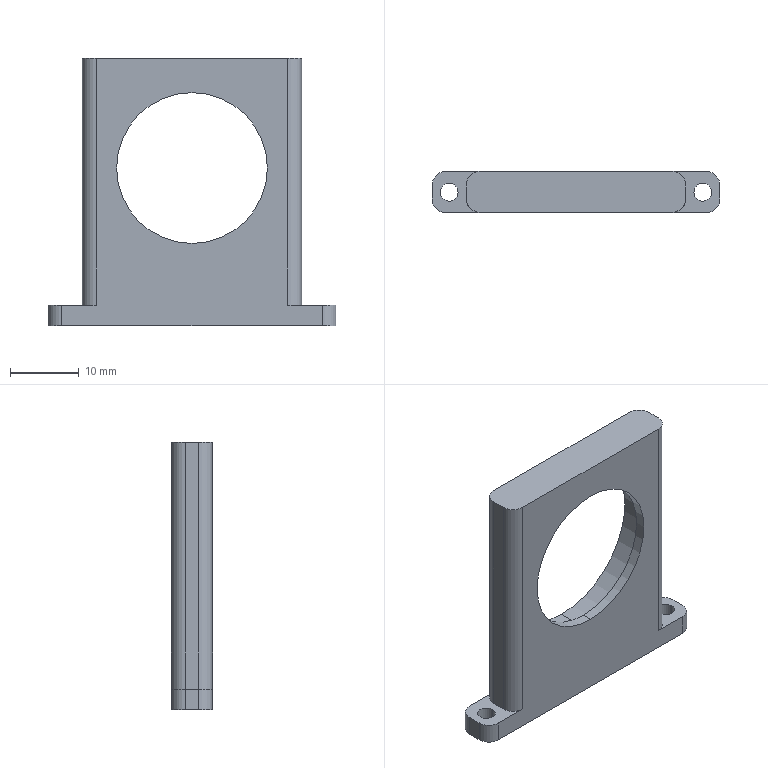NC program | NX | posted with a generic post | part box 42 x 6 x 39 mm
Whole program:
N10 G17 G21 G94 G90
(FLOOR_WALL_COPY , TOOL : D10JING)
N12 T14 M6
N14 G54
N16 G17 G0 G90 X-35. Y0. B0. C0. S6500 M3
N18 G43 Z30. H14
N20 Z3.
N22 G94 G1 Z0. F1500.
N24 X-30.
N26 X30.
N28 X35.
N30 Z3.
N32 G0 Z30.
N34 M5
(ADAPTIVE_MILLING , TOOL : D10)
N36 T15 M6
N38 G54
N40 G17 G0 G90 X-32.716 Y-0.772 B0. C0. S9500 M3
N42 G43 Z30. H15
N44 Z-17.
N46 G94 G1 Z-20. F1000.
N48 X-30.87 Y-0.608 F3000.
N50 G3 X-30.06 Y-0.061 R1.024
N52 X-29.299 Y3.003 R8.28
N54 G2 X-28.943 Y5.469 R10.893
N56 X-25.314 Y9.25 R6.938
N58 X-19.274 Y10.713 R17.09
N60 X-8.655 Y10.979 R140.997
N62 G1 X-6.03 Y10.984
N64 X-1.155 Y10.986
N66 X21.97 Y10.987
N68 X22.095 Y10.986
N70 X22.22 Y10.981
N72 X22.345 Y10.974
N74 G2 X26.605 Y8.207 R5.949
N76 X28.537 Y2.581 R13.213
N78 X28.903 Y-4.526 R46.257
N80 X25.999 Y-8.705 R6.102
N82 X20.346 Y-10.56 R13.549
N84 X11.111 Y-10.968 R78.805
N86 G1 X9.861 Y-10.974
N88 X7.986 Y-10.98
N90 X5.236 Y-10.984
N92 X-0.264 Y-10.987
N94 X-22.014
N96 X-22.139 Y-10.985
N98 G2 X-26.412 Y-8.474 R5.738
N100 X-28.455 Y-1.394 R11.572
N102 X-28.143 Y2.586 R19.594
N104 X-23.683 Y7.865 R8.373
N106 X-17.199 Y9.594 R18.267
N108 X-7.46 Y9.956 R104.445
N110 G1 X-5.835 Y9.964
N112 X-3.585 Y9.97
N114 X-0.46 Y9.974
N116 X6.165 Y9.976
N118 X18.915
N120 X19.04 Y9.975
N122 G2 X25.275 Y6.375 R7.621
N124 X27.448 Y0.044 R15.121
N126 X24.656 Y-6.884 R7.043
N128 X18.695 Y-9.312 R13.518
N130 X10.226 Y-9.922 R54.632
N132 G1 X9.476 Y-9.933
N134 X8.601 Y-9.943
N136 X7.476 Y-9.953
N138 X5.851 Y-9.962
N140 X4.226 Y-9.968
N142 X1.601 Y-9.973
N144 X-3.024 Y-9.975
N146 X-18.899 Y-9.976
N148 X-19.024 Y-9.975
N150 X-19.149 Y-9.972
N152 X-19.274 Y-9.967
N154 X-19.399 Y-9.961
N156 X-19.523 Y-9.952
N158 G2 X-25.728 Y-5.493 R7.674
N160 X-26.755 Y0.576 R10.359
N162 X-22.531 Y6.342 R8.556
N164 X-15.902 Y8.438 R17.454
N166 X-6.296 Y8.929 R81.762
N168 G1 X-5.171 Y8.939
N170 X-3.671 Y8.948
N172 X-1.921 Y8.955
N174 X0.579 Y8.961
N176 X4.579 Y8.964
N178 X15.204 Y8.965
N180 G2 X19.408 Y8.517 R12.623
N182 X24.833 Y3.457 R9.455
N184 X23.208 Y-5.189 R7.057
N186 X17.316 Y-8.05 R12.73
N188 X8.87 Y-8.874 R44.167
N190 X-5.88 Y-8.964 R738.817
N192 G1 X-16.255 Y-8.965
N194 X-16.505 Y-8.963
N196 X-16.63 Y-8.961
N198 X-16.755 Y-8.957
N200 X-16.88 Y-8.953
N202 X-17.129 Y-8.941
N204 G2 X-24.68 Y-2.319 R7.898
N206 X-21.942 Y4.208 R7.468
N208 X-18.99 Y6.066 R14.853
N210 G1 X-18.959 Y6.089
N212 X-18.5 Y6.548
N214 X-18.407 Y6.622
N216 G2 X-15.532 Y7.977 R8.149
N218 G1 X-14.03 Y8.147
N220 X-13.97 Y8.15
N222 X13.97
N224 G2 X19.21 Y6.907 R11.924
N226 X22.839 Y3.091 R7.696
N228 X21.487 Y-3.431 R6.455
N230 X19.943 Y-4.896 R22.468
N232 G1 X19.622 Y-5.407
N234 X19.548 Y-5.5
N236 G2 X15.647 Y-7.951 R7.671
N238 G1 X15.532 Y-7.977
N240 X14.03 Y-8.147
N242 X13.97 Y-8.15
N244 X-13.97
N246 G2 X-18.859 Y-7.029 R11.403
N248 X-21.442 Y0.444 R5.674
N250 G1 X-21.393 Y0.559
N252 X-21.343 Y0.673
N254 X-21.29 Y0.787
N256 X-21.236 Y0.899
N258 X-21.185 Y1.013
N260 X-21.145 Y1.132
N262 X-21.128 Y1.199
N264 G2 X-20.41 Y4.153 R7.86
N266 G1 X-19.622 Y5.407
N268 X-19.548 Y5.5
N270 X-18.929 Y6.119
N272 G3 X-19.262 Y7.753 R1.002
N274 X-20.138 Y7.714 Z-19.955 R1.174
N276 G1 X-21.183 Y7.371 Z-19.9
N278 X-22.764 Y6.853
N280 G3 X-23.429 Y6.119 R1.014
N282 G1 X-24.768 Y0.018
N284 X-24.918 Y-0.768
N286 X-25.052 Y-1.558
N288 G3 X-24.887 Y-3.645 R5.566
N290 X-24.04 Y-5.961 R10.729
N292 X-23.017 Y-7.495 R9.155
N294 G1 X-22.438 Y-8.191
N296 X-21.82 Y-8.855
N298 G3 X-19.157 Y-10.563 R8.253
N300 G1 X-17.212 Y-11.329
N302 G3 X-16.424 Y-11.305 R1.026
N304 G1 X-14.879 Y-10.586
N306 X-13.594 Y-9.977 Z-19.971
N308 G3 X-13.226 Y-9.542 Z-20. R1.052
N310 X-14.03 Y-8.147 R1.003
N312 G2 X-17.153 Y-7.41 R8.253
N314 X-20.41 Y-4.153 R7.671
N316 X-21.15 Y-0.97 R8.314
N318 X-21.119 Y1.278 R81.524
N320 G3 X-21.378 Y2.069 R1.024
N322 G1 X-21.768 Y2.491
N324 X-23.126 Y3.96 Z-19.9
N326 G2 X-23.369 Y5.175 R1.035
N328 G1 X-22.613 Y6.654
N330 G2 X-21.286 Y8.207 R6.058
N332 G1 X-19.93 Y9.308
N334 G2 X-17.059 Y10.738 R8.748
N336 X-15.22 Y11.007 R10.179
N338 X-11.481 Y11.184 R48.532
N340 G1 X10.848 Y11.329
N342 G2 X11.671 Y10.905 R1.015
N344 G1 X11.838 Y10.67
N346 X12.991 Y9.036 Z-20.
N348 X13.433 Y8.435
N350 G3 X14.03 Y8.147 R1.039
N352 G2 X17.153 Y7.41 R8.253
N354 X19.833 Y5.098 R7.737
N356 X20.977 Y2.532 R7.908
N358 X20.951 Y-2.647 R16.942
N360 G1 X20.462 Y-4.046
N362 X20.41 Y-4.153
N364 X19.878 Y-5.
N366 G3 X20.73 Y-6.532 R1.002
N368 X21.442 Y-6.254 Z-19.961 R1.197
N370 G1 X22.452 Y-5.568 Z-19.9
N372 X23.786 Y-4.662
N374 G3 X24.225 Y-3.835 R1.014
N376 G1 Y2.099
N378 G3 X23.612 Y5.107 R7.785
N380 G1 X23.281 Y5.903
N382 X22.926 Y6.69
N384 G3 X22.437 Y7.091 R1.042
N386 G1 X20.925 Y7.669
N388 X19.434 Y8.229 Z-19.98
N390 X19.232 Y8.251 Z-19.99
N392 X19.03 Y8.239 Z-20.
N394 G3 X18.5 Y6.548 R1.002
N396 G1 X19.548 Y5.5
N398 X19.622 Y5.407
N400 X20.087 Y4.667
N402 G3 X21.226 Y4.234 R1.017
N404 G1 X22.865 Y4.713
N406 Z-17.
N408 G0 Z30.
(ADAPTIVE_MILLING_COPY , TOOL : D10)
N410 X-32.718 Y-0.774
N412 Z-32.85
N414 G1 Z-35.85 F1000.
N416 X-30.872 Y-0.61 F3000.
N418 G3 X-30.061 Y-0.062 R1.024
N420 X-29.3 Y3.001 R8.28
N422 G2 X-28.945 Y5.468 R10.902
N424 X-25.315 Y9.248 R6.929
N426 X-19.4 Y10.7 R16.913
N428 X-8.032 Y10.982 R143.839
N430 G1 X-5.032 Y10.986
N432 X1.218 Y10.988
N434 X21.968
N436 X22.093 Y10.987
N438 X22.218 Y10.983
N440 X22.343 Y10.976
N442 G2 X26.46 Y8.414 R5.851
N444 X28.499 Y2.832 R12.663
N446 X28.904 Y-4.523 R46.026
N448 X26.111 Y-8.636 R6.036
N450 X20.353 Y-10.56 R13.48
N452 X11.618 Y-10.965 R74.55
N454 G1 X10.368 Y-10.973
N456 X8.743 Y-10.98
N458 X6.368 Y-10.985
N460 X2.368 Y-10.987
N462 X-14.882 Y-10.988
N464 X-22.007
N466 G2 X-26.333 Y-8.581 R5.647
N468 X-28.454 Y-1.403 R11.479
N470 X-28.146 Y2.578 R19.284
N472 X-23.691 Y7.859 R8.364
N474 X-16.959 Y9.621 R18.626
N476 X-6.594 Y9.962 R118.297
N478 G1 X-4.844 Y9.969
N480 X-2.344 Y9.974
N482 X1.906 Y9.977
N484 X17.406 Y9.978
N486 X18.906
N488 X19.031 Y9.977
N490 G2 X25.267 Y6.381 R7.606
N492 X27.448 Y0.052 R15.214
N494 X24.765 Y-6.801 R7.002
N496 X18.831 Y-9.288 R13.254
N498 X10.239 Y-9.923 R53.454
N500 G1 X9.49 Y-9.934
N502 X8.49 Y-9.946
N504 X7.24 Y-9.956
N506 X5.865 Y-9.964
N508 X3.865 Y-9.97
N510 X1.115 Y-9.975
N512 X-4.135 Y-9.977
N514 G2 X-19.634 Y-9.946 R874.968
N516 X-25.722 Y-5.511 R7.662
N518 X-26.781 Y0.433 R10.467
N520 X-22.44 Y6.395 R8.586
N522 X-15.549 Y8.483 R17.835
N524 X-4.94 Y8.943 R96.689
N526 G1 X-3.44 Y8.951
N528 X-1.44 Y8.958
N530 X1.31 Y8.963
N532 X5.935 Y8.966
N534 X16.31 Y8.967
N536 X16.435 Y8.966
N538 G2 X24.415 Y4.247 R8.919
N540 X25.651 Y-0.509 R7.89
N542 X22.053 Y-6.107 R7.807
N544 X15.375 Y-8.412 R15.908
N546 X5.896 Y-8.929 R76.575
N548 G1 X5.021 Y-8.938
N550 X3.646 Y-8.948
N552 X2.021 Y-8.955
N554 X-0.229 Y-8.961
N556 X-3.604 Y-8.965
N558 X-10.604 Y-8.967
N560 G2 X-17.478 Y-8.917 R150.563
N562 X-24.69 Y-2.226 R7.851
N564 X-22.058 Y4.104 R7.443
N566 X-19.014 Y6.047 R13.405
N568 X-17.046 Y7.462 R7.46
N570 X-13.97 Y8.15 R8.4
N572 G1 X13.97
N574 G2 X19.21 Y6.907 R11.909
N576 X22.84 Y3.092 R7.687
N578 X21.569 Y-3.334 R6.426
N580 X19.941 Y-4.9 R18.938
N582 G1 X19.622 Y-5.407
N584 X19.548 Y-5.5
N586 G2 X15.647 Y-7.951 R7.671
N588 G1 X15.532 Y-7.977
N590 X14.03 Y-8.147
N592 X13.97 Y-8.15
N594 X-13.97
N596 G2 X-18.859 Y-7.032 R11.377
N598 X-21.443 Y0.442 R5.676
N600 G1 X-21.394 Y0.556
N602 X-21.344 Y0.671
N604 X-21.291 Y0.784
N606 X-21.237 Y0.897
N608 X-21.185 Y1.011
N610 X-21.145 Y1.129
N612 X-21.128 Y1.199
N614 G2 X-20.41 Y4.153 R7.862
N616 G1 X-19.622 Y5.407
N618 X-19.548 Y5.5
N620 X-18.929 Y6.119
N622 G3 X-19.262 Y7.753 R1.002
N624 X-20.138 Y7.714 Z-35.805 R1.174
N626 G1 X-21.183 Y7.371 Z-35.75
N628 X-22.764 Y6.853
N630 G3 X-23.429 Y6.119 R1.014
N632 G1 X-24.768 Y0.018
N634 X-24.918 Y-0.768
N636 X-25.052 Y-1.558
N638 G3 X-24.887 Y-3.645 R5.566
N640 X-24.04 Y-5.961 R10.729
N642 X-23.017 Y-7.495 R9.155
N644 G1 X-22.438 Y-8.191
N646 X-21.82 Y-8.855
N648 G3 X-19.157 Y-10.563 R8.253
N650 G1 X-17.212 Y-11.329
N652 G3 X-16.424 Y-11.305 R1.026
N654 G1 X-14.879 Y-10.586
N656 X-13.594 Y-9.977 Z-35.821
N658 G3 X-13.226 Y-9.542 Z-35.85 R1.052
N660 X-14.03 Y-8.147 R1.003
N662 G2 X-17.153 Y-7.41 R8.253
N664 X-20.41 Y-4.153 R7.671
N666 X-21.15 Y-0.97 R8.314
N668 X-21.119 Y1.278 R81.524
N670 G3 X-21.378 Y2.069 R1.024
N672 G1 X-21.768 Y2.491
N674 X-23.126 Y3.96 Z-35.75
N676 G2 X-23.369 Y5.175 R1.035
N678 G1 X-22.613 Y6.654
N680 G2 X-21.286 Y8.207 R6.058
N682 G1 X-19.93 Y9.308
N684 G2 X-17.059 Y10.738 R8.748
N686 X-15.22 Y11.007 R10.179
N688 X-11.481 Y11.184 R48.532
N690 G1 X10.848 Y11.329
N692 G2 X11.671 Y10.905 R1.015
N694 G1 X11.838 Y10.67
N696 X12.991 Y9.036 Z-35.85
N698 X13.433 Y8.435
N700 G3 X14.03 Y8.147 R1.039
N702 G2 X17.153 Y7.41 R8.253
N704 X19.833 Y5.098 R7.737
N706 X20.977 Y2.532 R7.908
N708 X20.951 Y-2.647 R16.942
N710 G1 X20.462 Y-4.046
N712 X20.41 Y-4.153
N714 X19.878 Y-5.
N716 G3 X20.73 Y-6.532 R1.002
N718 X21.442 Y-6.254 Z-35.811 R1.197
N720 G1 X22.452 Y-5.568 Z-35.75
N722 X23.786 Y-4.662
N724 G3 X24.225 Y-3.835 R1.014
N726 G1 Y2.099
N728 G3 X23.612 Y5.107 R7.785
N730 G1 X23.281 Y5.903
N732 X22.926 Y6.69
N734 G3 X22.437 Y7.091 R1.042
N736 G1 X20.925 Y7.669
N738 X19.434 Y8.229 Z-35.83
N740 X19.232 Y8.251 Z-35.84
N742 X19.03 Y8.239 Z-35.85
N744 G3 X18.5 Y6.548 R1.002
N746 G1 X19.548 Y5.5
N748 X19.622 Y5.407
N750 X20.087 Y4.667
N752 G3 X21.226 Y4.234 R1.017
N754 G1 X22.865 Y4.713
N756 Z-32.85
N758 G0 Z30.
(ADAPTIVE_MILLING_COPY_COPY , TOOL : D10)
N760 X-32.709 Y-0.062
N762 Z-36.
N764 G1 Z-39. F1000.
N766 X-31.928 Y-0.342 F3000.
N768 X-31.14 Y-0.598
N770 G3 X-30.062 Y-0.062 R1.017
N772 X-29.3 Y3.001 R8.28
N774 G2 X-28.945 Y5.468 R10.902
N776 X-25.316 Y9.248 R6.931
N778 X-19.4 Y10.702 R17.009
N780 X-8.282 Y10.982 R140.28
N782 G1 X-5.407 Y10.986
N784 X0.343 Y10.988
N786 X21.968 Y10.989
N788 X22.093 Y10.988
N790 X22.218 Y10.983
N792 X22.342 Y10.976
N794 G2 X26.459 Y8.414 R5.853
N796 X28.499 Y2.832 R12.653
N798 X28.905 Y-4.522 R45.814
N800 X26.008 Y-8.705 R6.079
N802 X20.602 Y-10.528 R13.319
N804 X11.494 Y-10.967 R72.055
N806 G1 X10.244 Y-10.975
N808 X8.494 Y-10.981
N810 X5.994 Y-10.985
N812 X1.369 Y-10.988
N814 X-22.006 Y-10.989
N816 X-22.131 Y-10.987
N818 G2 X-26.406 Y-8.481 R5.736
N820 X-28.452 Y-1.153 R11.744
N822 X-28.147 Y2.577 R18.552
N824 X-23.692 Y7.859 R8.349
N826 X-17.085 Y9.608 R18.474
N828 X-6.095 Y9.965 R120.575
N830 G1 X-4.22 Y9.971
N832 X-1.47 Y9.975
N834 X3.655 Y9.977
N836 X18.905 Y9.978
N838 X19.03 Y9.977
N840 X19.154 Y9.974
N842 G2 X25.266 Y6.383 R7.619
N844 X27.452 Y0.055 R15.281
N846 X24.674 Y-6.879 R7.033
N848 X18.716 Y-9.313 R13.417
N850 X9.872 Y-9.929 R56.382
N852 G1 X8.873 Y-9.942
N854 X7.623 Y-9.954
N856 X6.248 Y-9.962
N858 X4.373 Y-9.969
N860 X1.873 Y-9.974
N862 X-2.502 Y-9.977
N864 G2 X-19.626 Y-9.947 R968.479
N866 X-25.772 Y-5.404 R7.688
N868 X-26.784 Y0.426 R10.437
N870 X-25.736 Y3.263 R7.883
N872 G1 X-25.462 Y4.046
N874 X-25.41 Y4.153
N876 G2 X-22.153 Y7.41 R7.671
N878 X-18.435 Y8.321 R12.433
N880 X-7.834 Y8.921 R86.583
N882 G1 X-6.709 Y8.933
N884 X-5.334 Y8.944
N886 X-3.709 Y8.952
N888 X-1.584 Y8.959
N890 X1.416 Y8.964
N892 X6.541 Y8.966
N894 G2 X17.29 Y8.932 R498.476
N896 X20.858 Y7.877 R8.597
N898 X23.5 Y6.548 R7.729
N900 X25.951 Y2.647 R7.671
N902 X26.15 Y0.005 R9.868
N904 X25.951 Y-2.647 R14.096
N906 X23.5 Y-6.548 R7.671
N908 X19.174 Y-8.197 R8.145
N910 X7.581 Y-8.921 R86.175
N912 G1 X6.456 Y-8.933
N914 X5.206 Y-8.943
N916 X3.581 Y-8.952
N918 X1.456 Y-8.959
N920 X-1.419 Y-8.963
N922 X-6.294 Y-8.966
N924 G2 X-17.293 Y-8.932 R561.239
N926 X-20.769 Y-7.908 R8.298
N928 X-23.5 Y-6.548 R7.88
N930 X-25.951 Y-2.647 R7.671
N932 X-25.951 Y2.647 R16.653
N934 G1 X-25.703 Y3.355
N936 X-25.566 Y3.758
N938 X-25.41 Y4.153
N940 G2 X-22.153 Y7.41 R7.671
N942 G1 X-22.046 Y7.462
N944 X-20.647 Y7.951
N946 X-20.532 Y7.977
N948 X-19.03 Y8.147
N950 X-18.97 Y8.15
N952 X18.97
N954 X19.03 Y8.147
N956 G2 X20.883 Y7.868 R8.601
N958 X23.5 Y6.548 R7.686
N960 X25.951 Y2.647 R7.671
N962 G1 X25.977 Y2.532
N964 X26.147 Y1.03
N966 X26.15 Y0.97
N968 Y-0.03
N970 G2 X25.951 Y-2.647 R14.051
N972 X23.5 Y-6.548 R7.671
N974 X20.532 Y-7.977 R8.027
N976 G1 X19.03 Y-8.147
N978 X18.97 Y-8.15
N980 X-18.97
N982 X-19.03 Y-8.147
N984 G2 X-20.883 Y-7.868 R8.601
N986 G3 X-22.184 Y-8.529 R1.014
N988 G1 X-22.603 Y-9.913
N990 Z-36.
N992 G0 Z30.
N994 M5
(ZLEVEL_PROFILE_COPY_1_COPY_COPY_1_COPY , TOOL : D10JING)
N996 T14 M6
N998 G54
N1000 G17 G0 G90 X15.645 Y-9.848 B0. C0. S9500 M3
N1002 G43 Z30. H14
N1004 Z-17.
N1006 G94 G1 Z-18. F1000.
N1008 X14.866 Y-8.5
N1010 G3 X14. Y-8. R1.
N1012 G1 X-14. F1200.
N1014 G2 X-21. Y-1. R7.
N1016 G1 Y1.
N1018 G2 X-14. Y8. R7.
N1020 G1 X14.
N1022 G2 X21. Y1. R7.
N1024 G1 Y-1.
N1026 G2 X14. Y-8. R7.
N1028 G3 X13.134 Y-8.5 R1.
N1030 G1 X12.268 Y-10.
N1032 Z-17.
N1034 G0 Z30.
N1036 X15.645 Y-9.848
N1038 Z-35.
N1040 G1 Z-36. F1000.
N1042 X14.866 Y-8.5
N1044 G3 X14. Y-8. R1.
N1046 G1 X-14. F1200.
N1048 G2 X-21. Y-1. R7.
N1050 G1 Y1.
N1052 G2 X-14. Y8. R7.
N1054 G1 X14.
N1056 G2 X21. Y1. R7.
N1058 G1 Y-1.
N1060 G2 X14. Y-8. R7.
N1062 G3 X13.134 Y-8.5 R1.
N1064 G1 X12.268 Y-10.
N1066 Z-35.
N1068 G0 Z30.
(ZLEVEL_PROFILE_COPY_1_COPY_COPY_1_COPY_COPY , TOOL : D10JING)
N1070 X-20.645 Y9.848
N1072 Z-38.
N1074 G1 Z-39. F1000.
N1076 X-19.866 Y8.5
N1078 G3 X-19. Y8. R1.
N1080 G1 X19. F1200.
N1082 G2 X26. Y1. R7.
N1084 G1 Y-1.
N1086 G2 X19. Y-8. R7.
N1088 G1 X-19.
N1090 G2 X-26. Y-1. R7.
N1092 G1 Y1.
N1094 G2 X-19. Y8. R7.
N1096 G3 X-18.134 Y8.5 R1.
N1098 G1 X-17.268 Y10.
N1100 Z-38.
N1102 G0 Z30.
N1104 M5
(PLANAR_MILL_COPY_COPY_COPY_COPY_COPY_COPY_1_COPY_1 , TOOL : D6A45)
N1106 T01 M6
N1108 G54
N1110 G17 G0 G90 X-1.27 Y5. B0. C0. S9500 M3
N1112 G43 Z30. H1
N1114 Z0.5
N1116 G94 G1 Z-1. F1250.
N1118 X-0.866 Y4.3
N1120 G3 X0. Y3.8 R1.
N1122 G1 X14.
N1124 G2 X16.8 Y1. R2.8
N1126 G1 Y-1.
N1128 G2 X14. Y-3.8 R2.8
N1130 G1 X-14.
N1132 G2 X-16.8 Y-1. R2.8
N1134 G1 Y1.
N1136 G2 X-14. Y3.8 R2.8
N1138 G1 X0.
N1140 G3 X0.866 Y4.3 R1.
N1142 G1 X1.27 Y5.
N1144 Z0.5
N1146 G0 Z30.
N1148 M5
(刀补14 , TOOL : D10JING)
N1150 T14 M6
N1152 G54
N1154 G17 G0 G90 X15.679 Y-9.942 B0. C0. S9500 M3
N1156 G43 Z30. H14
N1158 Z-17.
N1160 G94 G1 Z-18. F1000.
N1162 G41 X15.645 Y-9.848 D14
N1164 X14.866 Y-8.5
N1166 G3 X14. Y-8. R1.
N1168 G1 X-14. F1200.
N1170 G2 X-21. Y-1. R7.
N1172 G1 Y1.
N1174 G2 X-14. Y8. R7.
N1176 G1 X14.
N1178 G2 X21. Y1. R7.
N1180 G1 Y-1.
N1182 G2 X14. Y-8. R7.
N1184 G3 X13.134 Y-8.5 R1.
N1186 G1 X12.268 Y-10.
N1188 G40
N1190 X12.234 Y-10.094
N1192 Z-17.
N1194 G0 Z30.
N1196 X15.679 Y-9.942
N1198 Z-35.
N1200 G1 Z-36. F1000.
N1202 G41 X15.645 Y-9.848
N1204 X14.866 Y-8.5
N1206 G3 X14. Y-8. R1.
N1208 G1 X-14. F1200.
N1210 G2 X-21. Y-1. R7.
N1212 G1 Y1.
N1214 G2 X-14. Y8. R7.
N1216 G1 X14.
N1218 G2 X21. Y1. R7.
N1220 G1 Y-1.
N1222 G2 X14. Y-8. R7.
N1224 G3 X13.134 Y-8.5 R1.
N1226 G1 X12.268 Y-10.
N1228 G40
N1230 X12.234 Y-10.094
N1232 Z-35.
N1234 G0 Z30.
N1236 M5
N1238 M2